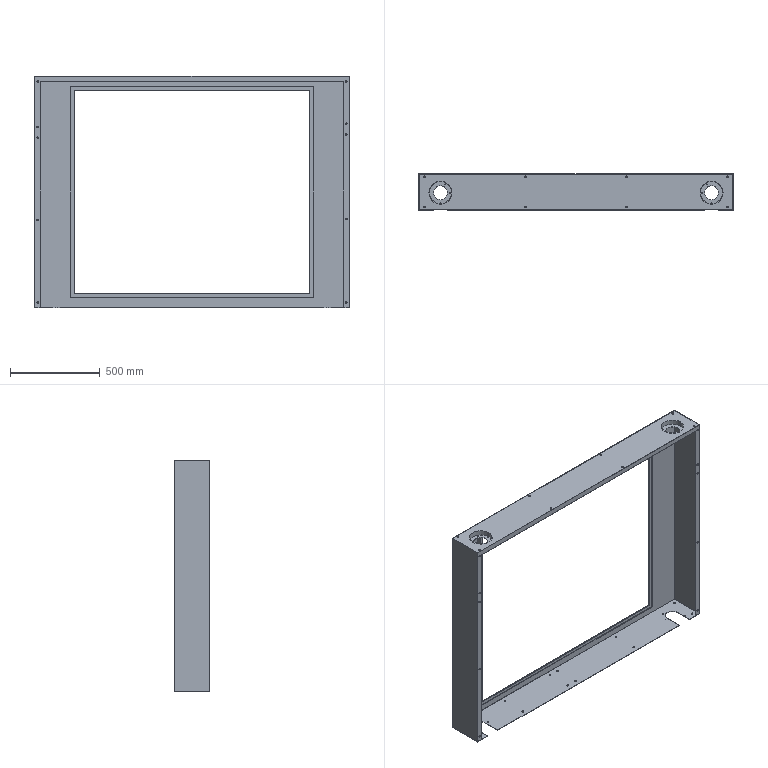Part | SolidWorks | features ICE 16, MirrorPattern 2, Extrusion 1, HoleWzd 1 | 1 solid | 136 faces | box 1750 x 200 x 1290 mm | volume 4398442 mm3 | cylinder 98 | plane 38 | commonest cylinder face diameters 9 x60 4.2 x24 78 x4 124 x4 128 x4 80 x2